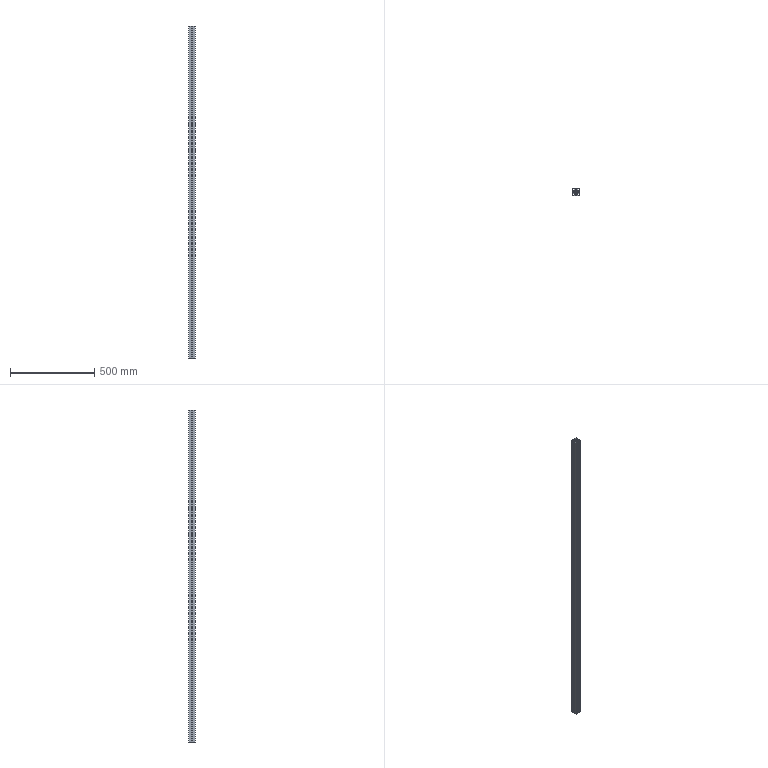Part | STEP file | 40_40_1350_1-2 | 1 solid | 64 faces | box 40 x 40 x 1970 mm | volume 1033744 mm3 | plane 62 | cylinder 2 | commonest cylinder face diameters 6.8 x2